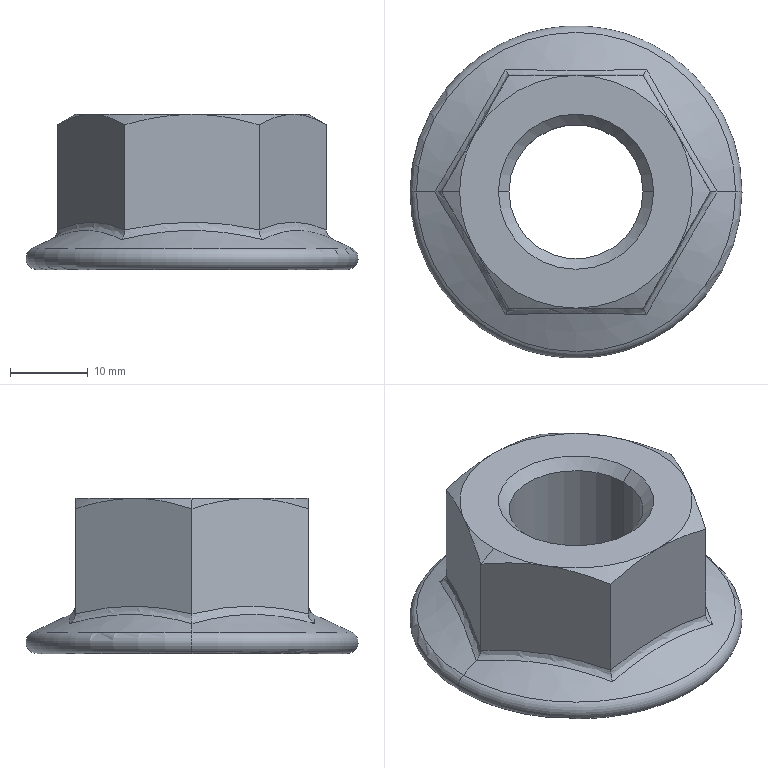Part | SolidWorks | features RevCut 3, Extrusion 1, Fillet 1, LPattern 1, Revolution 1 | 1 solid | 31 faces | box 42.8 x 42.8 x 20 mm | volume 13089 mm3 | cone 13 | plane 8 | spline 6 | torus 2 | cylinder 2 | commonest cylinder face diameters 17.294 x2
STEP:
#1=CARTESIAN_POINT('',(8.647,0.,-18.647));
#2=VERTEX_POINT('',#1);
#3=CARTESIAN_POINT('',(-8.647,0.,-18.647));
#4=VERTEX_POINT('',#3);
#5=CARTESIAN_POINT('',(0.,0.,-18.647));
#6=DIRECTION('',(0.,0.,-1.));
#7=DIRECTION('',(-1.,0.,0.));
#8=AXIS2_PLACEMENT_3D('',#5,#6,#7);
#9=CIRCLE('',#8,8.647);
#10=EDGE_CURVE('',#2,#4,#9,.T.);
#11=ORIENTED_EDGE('',*,*,#10,.F.);
#12=CARTESIAN_POINT('',(10.,0.,-20.));
#13=VERTEX_POINT('',#12);
#14=CARTESIAN_POINT('',(10.,0.,-20.));
#15=DIRECTION('',(0.7071,0.,-0.7071));
#16=VECTOR('',#15,1000.);
#17=LINE('',#14,#16);
#18=EDGE_CURVE('',#2,#13,#17,.T.);
#19=ORIENTED_EDGE('',*,*,#18,.T.);
#20=CARTESIAN_POINT('',(-10.,0.,-20.));
#21=VERTEX_POINT('',#20);
#22=CARTESIAN_POINT('',(0.,0.,-20.));
#23=DIRECTION('',(0.,0.,-1.));
#24=DIRECTION('',(-1.,0.,0.));
#25=AXIS2_PLACEMENT_3D('',#22,#23,#24);
#26=CIRCLE('',#25,10.);
#27=EDGE_CURVE('',#13,#21,#26,.T.);
#28=ORIENTED_EDGE('',*,*,#27,.T.);
#29=CARTESIAN_POINT('',(-10.,0.,-20.));
#30=DIRECTION('',(-0.7071,0.,-0.7071));
#31=VECTOR('',#30,1000.);
#32=LINE('',#29,#31);
#33=EDGE_CURVE('',#4,#21,#32,.T.);
#34=ORIENTED_EDGE('',*,*,#33,.F.);
#35=EDGE_LOOP('',(#11,#19,#28,#34));
#36=FACE_OUTER_BOUND('',#35,.T.);
#37=CARTESIAN_POINT('',(0.,0.,-20.));
#38=DIRECTION('',(0.,0.,-1.));
#39=DIRECTION('',(-1.,0.,0.));
#40=AXIS2_PLACEMENT_3D('',#37,#38,#39);
#41=CONICAL_SURFACE('',#40,10.,0.7854);
#42=ADVANCED_FACE('',(#36),#41,.F.);
#43=CARTESIAN_POINT('',(8.647,0.,-1.353));
#44=VERTEX_POINT('',#43);
#45=CARTESIAN_POINT('',(-8.647,0.,-1.353));
#46=VERTEX_POINT('',#45);
#47=CARTESIAN_POINT('',(0.,0.,-1.353));
#48=DIRECTION('',(0.,0.,-1.));
#49=DIRECTION('',(-1.,0.,0.));
#50=AXIS2_PLACEMENT_3D('',#47,#48,#49);
#51=CIRCLE('',#50,8.647);
#52=EDGE_CURVE('',#44,#46,#51,.T.);
#53=ORIENTED_EDGE('',*,*,#52,.T.);
#54=CARTESIAN_POINT('',(-10.,0.,0.));
#55=VERTEX_POINT('',#54);
#56=CARTESIAN_POINT('',(-8.647,0.,-1.353));
#57=DIRECTION('',(-0.7071,0.,0.7071));
#58=VECTOR('',#57,1000.);
#59=LINE('',#56,#58);
#60=EDGE_CURVE('',#46,#55,#59,.T.);
#61=ORIENTED_EDGE('',*,*,#60,.T.);
#62=CARTESIAN_POINT('',(10.,0.,0.));
#63=VERTEX_POINT('',#62);
#64=CARTESIAN_POINT('',(0.,0.,0.));
#65=DIRECTION('',(0.,0.,-1.));
#66=DIRECTION('',(-1.,0.,0.));
#67=AXIS2_PLACEMENT_3D('',#64,#65,#66);
#68=CIRCLE('',#67,10.);
#69=EDGE_CURVE('',#63,#55,#68,.T.);
#70=ORIENTED_EDGE('',*,*,#69,.F.);
#71=CARTESIAN_POINT('',(8.647,0.,-1.353));
#72=DIRECTION('',(0.7071,0.,0.7071));
#73=VECTOR('',#72,1000.);
#74=LINE('',#71,#73);
#75=EDGE_CURVE('',#44,#63,#74,.T.);
#76=ORIENTED_EDGE('',*,*,#75,.F.);
#77=EDGE_LOOP('',(#53,#61,#70,#76));
#78=FACE_OUTER_BOUND('',#77,.T.);
#79=CARTESIAN_POINT('',(0.,0.,-1.353));
#80=DIRECTION('',(0.,0.,1.));
#81=DIRECTION('',(1.,0.,0.));
#82=AXIS2_PLACEMENT_3D('',#79,#80,#81);
#83=CONICAL_SURFACE('',#82,8.647,0.7854);
#84=ADVANCED_FACE('',(#78),#83,.F.);
#85=CARTESIAN_POINT('',(9.1,15.761,-16.134));
#86=VERTEX_POINT('',#85);
#87=CARTESIAN_POINT('',(18.199,0.,-16.134));
#88=VERTEX_POINT('',#87);
#89=CARTESIAN_POINT('',(9.1,15.761,-16.134));
#90=CARTESIAN_POINT('',(9.83,14.459,-15.778));
#91=CARTESIAN_POINT('',(10.566,13.151,-15.485));
#92=CARTESIAN_POINT('',(12.056,10.52,-15.078));
#93=CARTESIAN_POINT('',(12.811,9.196,-14.966));
#94=CARTESIAN_POINT('',(13.965,7.198,-14.964));
#95=CARTESIAN_POINT('',(14.35,6.534,-14.991));
#96=CARTESIAN_POINT('',(15.123,5.21,-15.097));
#97=CARTESIAN_POINT('',(15.51,4.549,-15.177));
#98=CARTESIAN_POINT('',(16.668,2.582,-15.483));
#99=CARTESIAN_POINT('',(17.436,1.286,-15.778));
#100=CARTESIAN_POINT('',(18.199,0.,-16.134));
#101=B_SPLINE_CURVE_WITH_KNOTS('',3,(#89,#90,#91,#92,#93,#94,#95,#96,#97,#98,#99,#100),.UNSPECIFIED.,.F.,.F.,(4,2,2,2,2,4),(0.,0.004577,0.009154,0.01144,0.01373,0.01831),.UNSPECIFIED.);
#102=EDGE_CURVE('',#86,#88,#101,.T.);
#103=ORIENTED_EDGE('',*,*,#102,.T.);
#104=CARTESIAN_POINT('',(20.563,0.,-17.236));
#105=VERTEX_POINT('',#104);
#106=CARTESIAN_POINT('',(20.563,0.,-17.236));
#107=DIRECTION('',(0.9063,0.,-0.4226));
#108=VECTOR('',#107,1000.);
#109=LINE('',#106,#108);
#110=EDGE_CURVE('',#88,#105,#109,.T.);
#111=ORIENTED_EDGE('',*,*,#110,.T.);
#112=CARTESIAN_POINT('',(-20.563,0.,-17.236));
#113=VERTEX_POINT('',#112);
#114=CARTESIAN_POINT('',(0.,0.,-17.236));
#115=DIRECTION('',(0.,0.,1.));
#116=DIRECTION('',(1.,0.,0.));
#117=AXIS2_PLACEMENT_3D('',#114,#115,#116);
#118=CIRCLE('',#117,20.563);
#119=EDGE_CURVE('',#105,#113,#118,.T.);
#120=ORIENTED_EDGE('',*,*,#119,.T.);
#121=CARTESIAN_POINT('',(-18.199,0.,-16.134));
#122=VERTEX_POINT('',#121);
#123=CARTESIAN_POINT('',(-20.563,0.,-17.236));
#124=DIRECTION('',(-0.9063,0.,-0.4226));
#125=VECTOR('',#124,1000.);
#126=LINE('',#123,#125);
#127=EDGE_CURVE('',#122,#113,#126,.T.);
#128=ORIENTED_EDGE('',*,*,#127,.F.);
#129=CARTESIAN_POINT('',(-9.1,15.761,-16.134));
#130=VERTEX_POINT('',#129);
#131=CARTESIAN_POINT('',(-18.199,0.,-16.134));
#132=CARTESIAN_POINT('',(-17.437,1.284,-15.778));
#133=CARTESIAN_POINT('',(-16.672,2.575,-15.485));
#134=CARTESIAN_POINT('',(-15.138,5.181,-15.078));
#135=CARTESIAN_POINT('',(-14.37,6.497,-14.966));
#136=CARTESIAN_POINT('',(-13.216,8.495,-14.964));
#137=CARTESIAN_POINT('',(-12.834,9.161,-14.991));
#138=CARTESIAN_POINT('',(-12.073,10.492,-15.097));
#139=CARTESIAN_POINT('',(-11.695,11.157,-15.177));
#140=CARTESIAN_POINT('',(-10.57,13.144,-15.483));
#141=CARTESIAN_POINT('',(-9.832,14.457,-15.778));
#142=CARTESIAN_POINT('',(-9.1,15.761,-16.134));
#143=B_SPLINE_CURVE_WITH_KNOTS('',3,(#131,#132,#133,#134,#135,#136,#137,#138,#139,#140,#141,#142),.UNSPECIFIED.,.F.,.F.,(4,2,2,2,2,4),(0.,0.004577,0.009154,0.01144,0.01373,0.01831),.UNSPECIFIED.);
#144=EDGE_CURVE('',#122,#130,#143,.T.);
#145=ORIENTED_EDGE('',*,*,#144,.T.);
#146=CARTESIAN_POINT('',(-9.1,15.761,-16.134));
#147=CARTESIAN_POINT('',(-7.607,15.743,-15.778));
#148=CARTESIAN_POINT('',(-6.106,15.726,-15.485));
#149=CARTESIAN_POINT('',(-3.082,15.701,-15.078));
#150=CARTESIAN_POINT('',(-1.558,15.693,-14.966));
#151=CARTESIAN_POINT('',(0.749,15.693,-14.964));
#152=CARTESIAN_POINT('',(1.517,15.695,-14.991));
#153=CARTESIAN_POINT('',(3.05,15.702,-15.098));
#154=CARTESIAN_POINT('',(3.815,15.707,-15.177));
#155=CARTESIAN_POINT('',(6.098,15.726,-15.483));
#156=CARTESIAN_POINT('',(7.604,15.743,-15.778));
#157=CARTESIAN_POINT('',(9.1,15.761,-16.134));
#158=B_SPLINE_CURVE_WITH_KNOTS('',3,(#146,#147,#148,#149,#150,#151,#152,#153,#154,#155,#156,#157),.UNSPECIFIED.,.F.,.F.,(4,2,2,2,2,4),(0.,0.004577,0.009155,0.01144,0.01373,0.01831),.UNSPECIFIED.);
#159=EDGE_CURVE('',#130,#86,#158,.T.);
#160=ORIENTED_EDGE('',*,*,#159,.T.);
#161=EDGE_LOOP('',(#103,#111,#120,#128,#145,#160));
#162=FACE_OUTER_BOUND('',#161,.T.);
#163=CARTESIAN_POINT('',(0.,0.,-17.236));
#164=DIRECTION('',(0.,0.,-1.));
#165=DIRECTION('',(-1.,0.,0.));
#166=AXIS2_PLACEMENT_3D('',#163,#164,#165);
#167=CONICAL_SURFACE('',#166,20.563,1.134);
#168=ADVANCED_FACE('',(#162),#167,.T.);
#169=CARTESIAN_POINT('',(19.95,0.,-20.));
#170=VERTEX_POINT('',#169);
#171=CARTESIAN_POINT('',(-19.95,0.,-20.));
#172=VERTEX_POINT('',#171);
#173=CARTESIAN_POINT('',(0.,0.,-20.));
#174=DIRECTION('',(0.,0.,1.));
#175=DIRECTION('',(1.,0.,0.));
#176=AXIS2_PLACEMENT_3D('',#173,#174,#175);
#177=CIRCLE('',#176,19.95);
#178=EDGE_CURVE('',#170,#172,#177,.T.);
#179=ORIENTED_EDGE('',*,*,#178,.T.);
#180=CARTESIAN_POINT('',(-19.95,0.,-18.55));
#181=DIRECTION('',(0.,1.,0.));
#182=DIRECTION('',(-1.,0.,0.));
#183=AXIS2_PLACEMENT_3D('',#180,#181,#182);
#184=CIRCLE('',#183,1.45);
#185=EDGE_CURVE('',#172,#113,#184,.T.);
#186=ORIENTED_EDGE('',*,*,#185,.T.);
#187=ORIENTED_EDGE('',*,*,#119,.F.);
#188=CARTESIAN_POINT('',(19.95,0.,-18.55));
#189=DIRECTION('',(0.,-1.,0.));
#190=DIRECTION('',(0.,0.,-1.));
#191=AXIS2_PLACEMENT_3D('',#188,#189,#190);
#192=CIRCLE('',#191,1.45);
#193=EDGE_CURVE('',#170,#105,#192,.T.);
#194=ORIENTED_EDGE('',*,*,#193,.F.);
#195=EDGE_LOOP('',(#179,#186,#187,#194));
#196=FACE_OUTER_BOUND('',#195,.T.);
#197=CARTESIAN_POINT('',(0.,0.,-18.55));
#198=DIRECTION('',(0.,0.,1.));
#199=DIRECTION('',(1.,0.,0.));
#200=AXIS2_PLACEMENT_3D('',#197,#198,#199);
#201=TOROIDAL_SURFACE('',#200,19.95,1.45);
#202=ADVANCED_FACE('',(#196),#201,.T.);
#203=CARTESIAN_POINT('',(-15.,0.,0.));
#204=VERTEX_POINT('',#203);
#205=CARTESIAN_POINT('',(-12.99,-7.5,0.));
#206=VERTEX_POINT('',#205);
#207=CARTESIAN_POINT('',(0.,0.,0.));
#208=DIRECTION('',(0.,0.,1.));
#209=DIRECTION('',(-1.,0.,0.));
#210=AXIS2_PLACEMENT_3D('',#207,#208,#209);
#211=CIRCLE('',#210,15.);
#212=EDGE_CURVE('',#204,#206,#211,.T.);
#213=ORIENTED_EDGE('',*,*,#212,.F.);
#214=CARTESIAN_POINT('',(-17.321,0.,-1.34));
#215=VERTEX_POINT('',#214);
#216=CARTESIAN_POINT('',(-15.,0.,0.));
#217=DIRECTION('',(-0.866,0.,-0.5));
#218=VECTOR('',#217,1000.);
#219=LINE('',#216,#218);
#220=EDGE_CURVE('',#204,#215,#219,.T.);
#221=ORIENTED_EDGE('',*,*,#220,.T.);
#222=CARTESIAN_POINT('',(-17.321,0.,-1.34));
#223=CARTESIAN_POINT('',(-16.612,-1.227,-0.9308));
#224=CARTESIAN_POINT('',(-15.899,-2.463,-0.5939));
#225=CARTESIAN_POINT('',(-14.457,-4.96,-0.1277));
#226=CARTESIAN_POINT('',(-13.728,-6.222,0.));
#227=CARTESIAN_POINT('',(-12.99,-7.5,0.));
#228=B_SPLINE_CURVE_WITH_KNOTS('',3,(#222,#223,#224,#225,#226,#227),.UNSPECIFIED.,.F.,.F.,(4,2,4),(0.000000238,0.004382,0.008763),.UNSPECIFIED.);
#229=EDGE_CURVE('',#215,#206,#228,.T.);
#230=ORIENTED_EDGE('',*,*,#229,.T.);
#231=EDGE_LOOP('',(#213,#221,#230));
#232=FACE_OUTER_BOUND('',#231,.T.);
#233=CARTESIAN_POINT('',(0.,0.,0.));
#234=DIRECTION('',(0.,0.,-1.));
#235=DIRECTION('',(-1.,0.,0.));
#236=AXIS2_PLACEMENT_3D('',#233,#234,#235);
#237=CONICAL_SURFACE('',#236,15.,1.047);
#238=ADVANCED_FACE('',(#232),#237,.T.);
#239=ORIENTED_EDGE('',*,*,#10,.T.);
#240=CARTESIAN_POINT('',(-8.647,0.,-20.));
#241=DIRECTION('',(0.,0.,1.));
#242=VECTOR('',#241,1000.);
#243=LINE('',#240,#242);
#244=EDGE_CURVE('',#4,#46,#243,.T.);
#245=ORIENTED_EDGE('',*,*,#244,.T.);
#246=ORIENTED_EDGE('',*,*,#52,.F.);
#247=CARTESIAN_POINT('',(8.647,0.,-20.));
#248=DIRECTION('',(0.,0.,1.));
#249=VECTOR('',#248,1000.);
#250=LINE('',#247,#249);
#251=EDGE_CURVE('',#2,#44,#250,.T.);
#252=ORIENTED_EDGE('',*,*,#251,.F.);
#253=EDGE_LOOP('',(#239,#245,#246,#252));
#254=FACE_OUTER_BOUND('',#253,.T.);
#255=CARTESIAN_POINT('',(0.,0.,-20.));
#256=DIRECTION('',(0.,0.,1.));
#257=DIRECTION('',(1.,0.,0.));
#258=AXIS2_PLACEMENT_3D('',#255,#256,#257);
#259=CYLINDRICAL_SURFACE('',#258,8.647);
#260=ADVANCED_FACE('',(#254),#259,.F.);
#261=CARTESIAN_POINT('',(-8.66,-15.,-14.889));
#262=VERTEX_POINT('',#261);
#263=CARTESIAN_POINT('',(-8.66,-15.,-1.34));
#264=VERTEX_POINT('',#263);
#265=CARTESIAN_POINT('',(-8.66,-15.,-20.));
#266=DIRECTION('',(0.,0.,1.));
#267=VECTOR('',#266,1000.);
#268=LINE('',#265,#267);
#269=EDGE_CURVE('',#262,#264,#268,.T.);
#270=ORIENTED_EDGE('',*,*,#269,.F.);
#271=CARTESIAN_POINT('',(8.66,-15.,-14.889));
#272=VERTEX_POINT('',#271);
#273=CARTESIAN_POINT('',(-8.66,-15.,-14.889));
#274=CARTESIAN_POINT('',(-7.234,-15.,-14.575));
#275=CARTESIAN_POINT('',(-5.801,-15.,-14.321));
#276=CARTESIAN_POINT('',(-2.915,-15.,-13.971));
#277=CARTESIAN_POINT('',(-1.463,-15.,-13.877));
#278=CARTESIAN_POINT('',(1.463,-15.,-13.877));
#279=CARTESIAN_POINT('',(2.915,-15.,-13.971));
#280=CARTESIAN_POINT('',(5.801,-15.,-14.321));
#281=CARTESIAN_POINT('',(7.234,-15.,-14.575));
#282=CARTESIAN_POINT('',(8.66,-15.,-14.889));
#283=B_SPLINE_CURVE_WITH_KNOTS('',3,(#273,#274,#275,#276,#277,#278,#279,#280,#281,#282),.UNSPECIFIED.,.F.,.F.,(4,2,2,2,4),(0.,0.00436,0.008719,0.01308,0.01744),.UNSPECIFIED.);
#284=EDGE_CURVE('',#262,#272,#283,.T.);
#285=ORIENTED_EDGE('',*,*,#284,.T.);
#286=CARTESIAN_POINT('',(8.66,-15.,-1.34));
#287=VERTEX_POINT('',#286);
#288=CARTESIAN_POINT('',(8.66,-15.,-20.));
#289=DIRECTION('',(0.,0.,1.));
#290=VECTOR('',#289,1000.);
#291=LINE('',#288,#290);
#292=EDGE_CURVE('',#272,#287,#291,.T.);
#293=ORIENTED_EDGE('',*,*,#292,.T.);
#294=CARTESIAN_POINT('',(0.,-15.,0.));
#295=VERTEX_POINT('',#294);
#296=CARTESIAN_POINT('',(0.,-15.,0.));
#297=CARTESIAN_POINT('',(0.7322,-15.,0.));
#298=CARTESIAN_POINT('',(1.467,-15.,-0.03111));
#299=CARTESIAN_POINT('',(2.94,-15.,-0.1548));
#300=CARTESIAN_POINT('',(3.672,-15.,-0.2467));
#301=CARTESIAN_POINT('',(5.841,-15.,-0.5989));
#302=CARTESIAN_POINT('',(7.26,-15.,-0.9355));
#303=CARTESIAN_POINT('',(8.66,-15.,-1.34));
#304=B_SPLINE_CURVE_WITH_KNOTS('',3,(#296,#297,#298,#299,#300,#301,#302,#303),.UNSPECIFIED.,.F.,.F.,(4,2,2,4),(0.02421,0.0264,0.0286,0.03298),.UNSPECIFIED.);
#305=EDGE_CURVE('',#295,#287,#304,.T.);
#306=ORIENTED_EDGE('',*,*,#305,.F.);
#307=CARTESIAN_POINT('',(-8.66,-15.,-1.34));
#308=CARTESIAN_POINT('',(-7.956,-15.,-1.136));
#309=CARTESIAN_POINT('',(-7.245,-15.,-0.9498));
#310=CARTESIAN_POINT('',(-5.807,-15.,-0.6186));
#311=CARTESIAN_POINT('',(-5.086,-15.,-0.4755));
#312=CARTESIAN_POINT('',(-2.917,-15.,-0.1258));
#313=CARTESIAN_POINT('',(-1.463,-15.,0.));
#314=CARTESIAN_POINT('',(0.,-15.,0.));
#315=B_SPLINE_CURVE_WITH_KNOTS('',3,(#307,#308,#309,#310,#311,#312,#313,#314),.UNSPECIFIED.,.F.,.F.,(4,2,2,4),(0.01545,0.01764,0.01983,0.02421),.UNSPECIFIED.);
#316=EDGE_CURVE('',#264,#295,#315,.T.);
#317=ORIENTED_EDGE('',*,*,#316,.F.);
#318=EDGE_LOOP('',(#270,#285,#293,#306,#317));
#319=FACE_OUTER_BOUND('',#318,.T.);
#320=CARTESIAN_POINT('',(-8.66,-15.,-20.));
#321=DIRECTION('',(0.,-1.,0.));
#322=DIRECTION('',(1.,0.,0.));
#323=AXIS2_PLACEMENT_3D('',#320,#321,#322);
#324=PLANE('',#323);
#325=ADVANCED_FACE('',(#319),#324,.T.);
#326=CARTESIAN_POINT('',(-17.321,0.,-14.889));
#327=VERTEX_POINT('',#326);
#328=CARTESIAN_POINT('',(-17.321,0.,-20.));
#329=DIRECTION('',(0.,0.,1.));
#330=VECTOR('',#329,1000.);
#331=LINE('',#328,#330);
#332=EDGE_CURVE('',#327,#215,#331,.T.);
#333=ORIENTED_EDGE('',*,*,#332,.F.);
#334=CARTESIAN_POINT('',(-17.321,0.,-14.889));
#335=CARTESIAN_POINT('',(-16.607,-1.235,-14.575));
#336=CARTESIAN_POINT('',(-15.891,-2.477,-14.321));
#337=CARTESIAN_POINT('',(-14.448,-4.976,-13.971));
#338=CARTESIAN_POINT('',(-13.722,-6.234,-13.877));
#339=CARTESIAN_POINT('',(-12.259,-8.767,-13.877));
#340=CARTESIAN_POINT('',(-11.533,-10.025,-13.971));
#341=CARTESIAN_POINT('',(-10.09,-12.523,-14.321));
#342=CARTESIAN_POINT('',(-9.373,-13.765,-14.575));
#343=CARTESIAN_POINT('',(-8.66,-15.,-14.889));
#344=B_SPLINE_CURVE_WITH_KNOTS('',3,(#334,#335,#336,#337,#338,#339,#340,#341,#342,#343),.UNSPECIFIED.,.F.,.F.,(4,2,2,2,4),(0.,0.00436,0.00872,0.01308,0.01744),.UNSPECIFIED.);
#345=EDGE_CURVE('',#327,#262,#344,.T.);
#346=ORIENTED_EDGE('',*,*,#345,.T.);
#347=ORIENTED_EDGE('',*,*,#269,.T.);
#348=CARTESIAN_POINT('',(-12.99,-7.5,0.));
#349=CARTESIAN_POINT('',(-12.623,-8.136,0.));
#350=CARTESIAN_POINT('',(-12.254,-8.776,-0.03167));
#351=CARTESIAN_POINT('',(-11.524,-10.041,-0.1542));
#352=CARTESIAN_POINT('',(-11.161,-10.669,-0.245));
#353=CARTESIAN_POINT('',(-10.079,-12.542,-0.595));
#354=CARTESIAN_POINT('',(-9.367,-13.776,-0.9318));
#355=CARTESIAN_POINT('',(-8.66,-15.,-1.34));
#356=B_SPLINE_CURVE_WITH_KNOTS('',3,(#348,#349,#350,#351,#352,#353,#354,#355),.UNSPECIFIED.,.F.,.F.,(4,2,2,4),(0.008763,0.01095,0.01313,0.01749),.UNSPECIFIED.);
#357=EDGE_CURVE('',#206,#264,#356,.T.);
#358=ORIENTED_EDGE('',*,*,#357,.F.);
#359=ORIENTED_EDGE('',*,*,#229,.F.);
#360=EDGE_LOOP('',(#333,#346,#347,#358,#359));
#361=FACE_OUTER_BOUND('',#360,.T.);
#362=CARTESIAN_POINT('',(-17.321,0.,-20.));
#363=DIRECTION('',(-0.866,-0.5,0.));
#364=DIRECTION('',(0.5,-0.866,0.));
#365=AXIS2_PLACEMENT_3D('',#362,#363,#364);
#366=PLANE('',#365);
#367=ADVANCED_FACE('',(#361),#366,.T.);
#368=CARTESIAN_POINT('',(-8.66,15.,-14.889));
#369=VERTEX_POINT('',#368);
#370=CARTESIAN_POINT('',(-8.66,15.,-1.34));
#371=VERTEX_POINT('',#370);
#372=CARTESIAN_POINT('',(-8.66,15.,-20.));
#373=DIRECTION('',(0.,0.,1.));
#374=VECTOR('',#373,1000.);
#375=LINE('',#372,#374);
#376=EDGE_CURVE('',#369,#371,#375,.T.);
#377=ORIENTED_EDGE('',*,*,#376,.F.);
#378=CARTESIAN_POINT('',(-8.66,15.,-14.889));
#379=CARTESIAN_POINT('',(-9.373,13.765,-14.575));
#380=CARTESIAN_POINT('',(-10.09,12.523,-14.321));
#381=CARTESIAN_POINT('',(-11.533,10.024,-13.971));
#382=CARTESIAN_POINT('',(-12.259,8.766,-13.877));
#383=CARTESIAN_POINT('',(-13.722,6.233,-13.877));
#384=CARTESIAN_POINT('',(-14.448,4.975,-13.971));
#385=CARTESIAN_POINT('',(-15.891,2.477,-14.321));
#386=CARTESIAN_POINT('',(-16.607,1.235,-14.575));
#387=CARTESIAN_POINT('',(-17.321,0.,-14.889));
#388=B_SPLINE_CURVE_WITH_KNOTS('',3,(#378,#379,#380,#381,#382,#383,#384,#385,#386,#387),.UNSPECIFIED.,.F.,.F.,(4,2,2,2,4),(0.,0.00436,0.00872,0.01308,0.01744),.UNSPECIFIED.);
#389=EDGE_CURVE('',#369,#327,#388,.T.);
#390=ORIENTED_EDGE('',*,*,#389,.T.);
#391=ORIENTED_EDGE('',*,*,#332,.T.);
#392=CARTESIAN_POINT('',(-12.99,7.5,0.));
#393=VERTEX_POINT('',#392);
#394=CARTESIAN_POINT('',(-12.99,7.5,0.));
#395=CARTESIAN_POINT('',(-13.358,6.864,0.));
#396=CARTESIAN_POINT('',(-13.727,6.224,-0.03167));
#397=CARTESIAN_POINT('',(-14.457,4.959,-0.1542));
#398=CARTESIAN_POINT('',(-14.82,4.331,-0.245));
#399=CARTESIAN_POINT('',(-15.901,2.458,-0.595));
#400=CARTESIAN_POINT('',(-16.614,1.224,-0.9318));
#401=CARTESIAN_POINT('',(-17.321,0.,-1.34));
#402=B_SPLINE_CURVE_WITH_KNOTS('',3,(#394,#395,#396,#397,#398,#399,#400,#401),.UNSPECIFIED.,.F.,.F.,(4,2,2,4),(0.008763,0.01095,0.01313,0.01749),.UNSPECIFIED.);
#403=EDGE_CURVE('',#393,#215,#402,.T.);
#404=ORIENTED_EDGE('',*,*,#403,.F.);
#405=CARTESIAN_POINT('',(-8.66,15.,-1.34));
#406=CARTESIAN_POINT('',(-9.369,13.773,-0.9308));
#407=CARTESIAN_POINT('',(-10.082,12.537,-0.5939));
#408=CARTESIAN_POINT('',(-11.524,10.04,-0.1277));
#409=CARTESIAN_POINT('',(-12.253,8.778,0.));
#410=CARTESIAN_POINT('',(-12.99,7.5,0.));
#411=B_SPLINE_CURVE_WITH_KNOTS('',3,(#405,#406,#407,#408,#409,#410),.UNSPECIFIED.,.F.,.F.,(4,2,4),(0.000000238,0.004382,0.008763),.UNSPECIFIED.);
#412=EDGE_CURVE('',#371,#393,#411,.T.);
#413=ORIENTED_EDGE('',*,*,#412,.F.);
#414=EDGE_LOOP('',(#377,#390,#391,#404,#413));
#415=FACE_OUTER_BOUND('',#414,.T.);
#416=CARTESIAN_POINT('',(-8.66,15.,-20.));
#417=DIRECTION('',(-0.866,0.5,0.));
#418=DIRECTION('',(-0.5,-0.866,0.));
#419=AXIS2_PLACEMENT_3D('',#416,#417,#418);
#420=PLANE('',#419);
#421=ADVANCED_FACE('',(#415),#420,.T.);
#422=CARTESIAN_POINT('',(8.66,15.,-14.889));
#423=VERTEX_POINT('',#422);
#424=CARTESIAN_POINT('',(8.66,15.,-1.34));
#425=VERTEX_POINT('',#424);
#426=CARTESIAN_POINT('',(8.66,15.,-20.));
#427=DIRECTION('',(0.,0.,1.));
#428=VECTOR('',#427,1000.);
#429=LINE('',#426,#428);
#430=EDGE_CURVE('',#423,#425,#429,.T.);
#431=ORIENTED_EDGE('',*,*,#430,.F.);
#432=CARTESIAN_POINT('',(8.66,15.,-14.889));
#433=CARTESIAN_POINT('',(7.234,15.,-14.575));
#434=CARTESIAN_POINT('',(5.801,15.,-14.321));
#435=CARTESIAN_POINT('',(2.915,15.,-13.971));
#436=CARTESIAN_POINT('',(1.463,15.,-13.877));
#437=CARTESIAN_POINT('',(-1.463,15.,-13.877));
#438=CARTESIAN_POINT('',(-2.915,15.,-13.971));
#439=CARTESIAN_POINT('',(-5.801,15.,-14.321));
#440=CARTESIAN_POINT('',(-7.234,15.,-14.575));
#441=CARTESIAN_POINT('',(-8.66,15.,-14.889));
#442=B_SPLINE_CURVE_WITH_KNOTS('',3,(#432,#433,#434,#435,#436,#437,#438,#439,#440,#441),.UNSPECIFIED.,.F.,.F.,(4,2,2,2,4),(0.,0.00436,0.008719,0.01308,0.01744),.UNSPECIFIED.);
#443=EDGE_CURVE('',#423,#369,#442,.T.);
#444=ORIENTED_EDGE('',*,*,#443,.T.);
#445=ORIENTED_EDGE('',*,*,#376,.T.);
#446=CARTESIAN_POINT('',(0.,15.,0.));
#447=VERTEX_POINT('',#446);
#448=CARTESIAN_POINT('',(0.,15.,0.));
#449=CARTESIAN_POINT('',(-1.463,15.,0.));
#450=CARTESIAN_POINT('',(-2.917,15.,-0.1258));
#451=CARTESIAN_POINT('',(-5.086,15.,-0.4755));
#452=CARTESIAN_POINT('',(-5.807,15.,-0.6186));
#453=CARTESIAN_POINT('',(-7.245,15.,-0.9498));
#454=CARTESIAN_POINT('',(-7.956,15.,-1.136));
#455=CARTESIAN_POINT('',(-8.66,15.,-1.34));
#456=B_SPLINE_CURVE_WITH_KNOTS('',3,(#448,#449,#450,#451,#452,#453,#454,#455),.UNSPECIFIED.,.F.,.F.,(4,2,2,4),(0.01509,0.01946,0.02165,0.02383),.UNSPECIFIED.);
#457=EDGE_CURVE('',#447,#371,#456,.T.);
#458=ORIENTED_EDGE('',*,*,#457,.F.);
#459=CARTESIAN_POINT('',(8.66,15.,-1.34));
#460=CARTESIAN_POINT('',(7.26,15.,-0.9355));
#461=CARTESIAN_POINT('',(5.841,15.,-0.5989));
#462=CARTESIAN_POINT('',(3.672,15.,-0.2467));
#463=CARTESIAN_POINT('',(2.94,15.,-0.1548));
#464=CARTESIAN_POINT('',(1.467,15.,-0.03111));
#465=CARTESIAN_POINT('',(0.7322,15.,0.));
#466=CARTESIAN_POINT('',(0.,15.,0.));
#467=B_SPLINE_CURVE_WITH_KNOTS('',3,(#459,#460,#461,#462,#463,#464,#465,#466),.UNSPECIFIED.,.F.,.F.,(4,2,2,4),(0.006348,0.01072,0.01291,0.01509),.UNSPECIFIED.);
#468=EDGE_CURVE('',#425,#447,#467,.T.);
#469=ORIENTED_EDGE('',*,*,#468,.F.);
#470=EDGE_LOOP('',(#431,#444,#445,#458,#469));
#471=FACE_OUTER_BOUND('',#470,.T.);
#472=CARTESIAN_POINT('',(8.66,15.,-20.));
#473=DIRECTION('',(0.,1.,0.));
#474=DIRECTION('',(-1.,0.,0.));
#475=AXIS2_PLACEMENT_3D('',#472,#473,#474);
#476=PLANE('',#475);
#477=ADVANCED_FACE('',(#471),#476,.T.);
#478=CARTESIAN_POINT('',(17.321,0.,-14.889));
#479=VERTEX_POINT('',#478);
#480=CARTESIAN_POINT('',(17.321,0.,-1.34));
#481=VERTEX_POINT('',#480);
#482=CARTESIAN_POINT('',(17.321,0.,-20.));
#483=DIRECTION('',(0.,0.,1.));
#484=VECTOR('',#483,1000.);
#485=LINE('',#482,#484);
#486=EDGE_CURVE('',#479,#481,#485,.T.);
#487=ORIENTED_EDGE('',*,*,#486,.F.);
#488=CARTESIAN_POINT('',(17.321,0.,-14.889));
#489=CARTESIAN_POINT('',(16.607,1.235,-14.575));
#490=CARTESIAN_POINT('',(15.891,2.477,-14.321));
#491=CARTESIAN_POINT('',(14.448,4.976,-13.971));
#492=CARTESIAN_POINT('',(13.722,6.234,-13.877));
#493=CARTESIAN_POINT('',(12.259,8.767,-13.877));
#494=CARTESIAN_POINT('',(11.533,10.025,-13.971));
#495=CARTESIAN_POINT('',(10.09,12.523,-14.321));
#496=CARTESIAN_POINT('',(9.373,13.765,-14.575));
#497=CARTESIAN_POINT('',(8.66,15.,-14.889));
#498=B_SPLINE_CURVE_WITH_KNOTS('',3,(#488,#489,#490,#491,#492,#493,#494,#495,#496,#497),.UNSPECIFIED.,.F.,.F.,(4,2,2,2,4),(0.,0.00436,0.00872,0.01308,0.01744),.UNSPECIFIED.);
#499=EDGE_CURVE('',#479,#423,#498,.T.);
#500=ORIENTED_EDGE('',*,*,#499,.T.);
#501=ORIENTED_EDGE('',*,*,#430,.T.);
#502=CARTESIAN_POINT('',(12.99,7.5,0.));
#503=VERTEX_POINT('',#502);
#504=CARTESIAN_POINT('',(12.99,7.5,0.));
#505=CARTESIAN_POINT('',(12.623,8.136,0.));
#506=CARTESIAN_POINT('',(12.254,8.776,-0.03167));
#507=CARTESIAN_POINT('',(11.524,10.041,-0.1542));
#508=CARTESIAN_POINT('',(11.161,10.669,-0.245));
#509=CARTESIAN_POINT('',(10.079,12.542,-0.595));
#510=CARTESIAN_POINT('',(9.367,13.776,-0.9318));
#511=CARTESIAN_POINT('',(8.66,15.,-1.34));
#512=B_SPLINE_CURVE_WITH_KNOTS('',3,(#504,#505,#506,#507,#508,#509,#510,#511),.UNSPECIFIED.,.F.,.F.,(4,2,2,4),(0.008763,0.01095,0.01313,0.01749),.UNSPECIFIED.);
#513=EDGE_CURVE('',#503,#425,#512,.T.);
#514=ORIENTED_EDGE('',*,*,#513,.F.);
#515=CARTESIAN_POINT('',(17.321,0.,-1.34));
#516=CARTESIAN_POINT('',(16.612,1.227,-0.9308));
#517=CARTESIAN_POINT('',(15.899,2.463,-0.5939));
#518=CARTESIAN_POINT('',(14.457,4.96,-0.1277));
#519=CARTESIAN_POINT('',(13.728,6.222,0.));
#520=CARTESIAN_POINT('',(12.99,7.5,0.));
#521=B_SPLINE_CURVE_WITH_KNOTS('',3,(#515,#516,#517,#518,#519,#520),.UNSPECIFIED.,.F.,.F.,(4,2,4),(0.000000238,0.004382,0.008763),.UNSPECIFIED.);
#522=EDGE_CURVE('',#481,#503,#521,.T.);
#523=ORIENTED_EDGE('',*,*,#522,.F.);
#524=EDGE_LOOP('',(#487,#500,#501,#514,#523));
#525=FACE_OUTER_BOUND('',#524,.T.);
#526=CARTESIAN_POINT('',(17.321,0.,-20.));
#527=DIRECTION('',(0.866,0.5,0.));
#528=DIRECTION('',(-0.5,0.866,0.));
#529=AXIS2_PLACEMENT_3D('',#526,#527,#528);
#530=PLANE('',#529);
#531=ADVANCED_FACE('',(#525),#530,.T.);
#532=ORIENTED_EDGE('',*,*,#292,.F.);
#533=CARTESIAN_POINT('',(8.66,-15.,-14.889));
#534=CARTESIAN_POINT('',(9.373,-13.765,-14.575));
#535=CARTESIAN_POINT('',(10.09,-12.523,-14.321));
#536=CARTESIAN_POINT('',(11.533,-10.024,-13.971));
#537=CARTESIAN_POINT('',(12.259,-8.766,-13.877));
#538=CARTESIAN_POINT('',(13.722,-6.233,-13.877));
#539=CARTESIAN_POINT('',(14.448,-4.975,-13.971));
#540=CARTESIAN_POINT('',(15.891,-2.477,-14.321));
#541=CARTESIAN_POINT('',(16.607,-1.235,-14.575));
#542=CARTESIAN_POINT('',(17.321,0.,-14.889));
#543=B_SPLINE_CURVE_WITH_KNOTS('',3,(#533,#534,#535,#536,#537,#538,#539,#540,#541,#542),.UNSPECIFIED.,.F.,.F.,(4,2,2,2,4),(0.,0.00436,0.00872,0.01308,0.01744),.UNSPECIFIED.);
#544=EDGE_CURVE('',#272,#479,#543,.T.);
#545=ORIENTED_EDGE('',*,*,#544,.T.);
#546=ORIENTED_EDGE('',*,*,#486,.T.);
#547=CARTESIAN_POINT('',(12.99,-7.5,0.));
#548=VERTEX_POINT('',#547);
#549=CARTESIAN_POINT('',(12.99,-7.5,0.));
#550=CARTESIAN_POINT('',(13.358,-6.864,0.));
#551=CARTESIAN_POINT('',(13.727,-6.224,-0.03167));
#552=CARTESIAN_POINT('',(14.457,-4.959,-0.1542));
#553=CARTESIAN_POINT('',(14.82,-4.331,-0.245));
#554=CARTESIAN_POINT('',(15.901,-2.458,-0.595));
#555=CARTESIAN_POINT('',(16.614,-1.224,-0.9318));
#556=CARTESIAN_POINT('',(17.321,0.,-1.34));
#557=B_SPLINE_CURVE_WITH_KNOTS('',3,(#549,#550,#551,#552,#553,#554,#555,#556),.UNSPECIFIED.,.F.,.F.,(4,2,2,4),(0.008763,0.01095,0.01313,0.01749),.UNSPECIFIED.);
#558=EDGE_CURVE('',#548,#481,#557,.T.);
#559=ORIENTED_EDGE('',*,*,#558,.F.);
#560=CARTESIAN_POINT('',(8.66,-15.,-1.34));
#561=CARTESIAN_POINT('',(9.369,-13.773,-0.9308));
#562=CARTESIAN_POINT('',(10.082,-12.537,-0.5939));
#563=CARTESIAN_POINT('',(11.524,-10.04,-0.1277));
#564=CARTESIAN_POINT('',(12.253,-8.778,0.));
#565=CARTESIAN_POINT('',(12.99,-7.5,0.));
#566=B_SPLINE_CURVE_WITH_KNOTS('',3,(#560,#561,#562,#563,#564,#565),.UNSPECIFIED.,.F.,.F.,(4,2,4),(0.000000238,0.004382,0.008763),.UNSPECIFIED.);
#567=EDGE_CURVE('',#287,#548,#566,.T.);
#568=ORIENTED_EDGE('',*,*,#567,.F.);
#569=EDGE_LOOP('',(#532,#545,#546,#559,#568));
#570=FACE_OUTER_BOUND('',#569,.T.);
#571=CARTESIAN_POINT('',(8.66,-15.,-20.));
#572=DIRECTION('',(0.866,-0.5,0.));
#573=DIRECTION('',(0.5,0.866,0.));
#574=AXIS2_PLACEMENT_3D('',#571,#572,#573);
#575=PLANE('',#574);
#576=ADVANCED_FACE('',(#570),#575,.T.);
#577=CARTESIAN_POINT('',(0.,0.,-20.));
#578=DIRECTION('',(0.,0.,-1.));
#579=DIRECTION('',(-1.,0.,0.));
#580=AXIS2_PLACEMENT_3D('',#577,#578,#579);
#581=CIRCLE('',#580,10.);
#582=EDGE_CURVE('',#21,#13,#581,.T.);
#583=ORIENTED_EDGE('',*,*,#582,.F.);
#584=ORIENTED_EDGE('',*,*,#27,.F.);
#585=EDGE_LOOP('',(#583,#584));
#586=FACE_BOUND('',#585,.T.);
#587=ORIENTED_EDGE('',*,*,#178,.F.);
#588=CARTESIAN_POINT('',(0.,0.,-20.));
#589=DIRECTION('',(0.,0.,1.));
#590=DIRECTION('',(1.,0.,0.));
#591=AXIS2_PLACEMENT_3D('',#588,#589,#590);
#592=CIRCLE('',#591,19.95);
#593=EDGE_CURVE('',#172,#170,#592,.T.);
#594=ORIENTED_EDGE('',*,*,#593,.F.);
#595=EDGE_LOOP('',(#587,#594));
#596=FACE_OUTER_BOUND('',#595,.T.);
#597=CARTESIAN_POINT('',(-25.981,-15.,-20.));
#598=DIRECTION('',(0.,0.,-1.));
#599=DIRECTION('',(-1.,0.,0.));
#600=AXIS2_PLACEMENT_3D('',#597,#598,#599);
#601=PLANE('',#600);
#602=ADVANCED_FACE('',(#586,#596),#601,.T.);
#603=ORIENTED_EDGE('',*,*,#69,.T.);
#604=CARTESIAN_POINT('',(0.,0.,0.));
#605=DIRECTION('',(0.,0.,-1.));
#606=DIRECTION('',(-1.,0.,0.));
#607=AXIS2_PLACEMENT_3D('',#604,#605,#606);
#608=CIRCLE('',#607,10.);
#609=EDGE_CURVE('',#55,#63,#608,.T.);
#610=ORIENTED_EDGE('',*,*,#609,.T.);
#611=EDGE_LOOP('',(#603,#610));
#612=FACE_BOUND('',#611,.T.);
#613=CARTESIAN_POINT('',(0.,0.,0.));
#614=DIRECTION('',(0.,0.,1.));
#615=DIRECTION('',(-1.,0.,0.));
#616=AXIS2_PLACEMENT_3D('',#613,#614,#615);
#617=CIRCLE('',#616,15.);
#618=EDGE_CURVE('',#393,#204,#617,.T.);
#619=ORIENTED_EDGE('',*,*,#618,.T.);
#620=ORIENTED_EDGE('',*,*,#212,.T.);
#621=CARTESIAN_POINT('',(0.,0.,0.));
#622=DIRECTION('',(0.,0.,1.));
#623=DIRECTION('',(-1.,0.,0.));
#624=AXIS2_PLACEMENT_3D('',#621,#622,#623);
#625=CIRCLE('',#624,15.);
#626=EDGE_CURVE('',#206,#295,#625,.T.);
#627=ORIENTED_EDGE('',*,*,#626,.T.);
#628=CARTESIAN_POINT('',(0.,0.,0.));
#629=DIRECTION('',(0.,0.,1.));
#630=DIRECTION('',(-1.,0.,0.));
#631=AXIS2_PLACEMENT_3D('',#628,#629,#630);
#632=CIRCLE('',#631,15.);
#633=EDGE_CURVE('',#295,#548,#632,.T.);
#634=ORIENTED_EDGE('',*,*,#633,.T.);
#635=CARTESIAN_POINT('',(0.,0.,0.));
#636=DIRECTION('',(0.,0.,1.));
#637=DIRECTION('',(-1.,0.,0.));
#638=AXIS2_PLACEMENT_3D('',#635,#636,#637);
#639=CIRCLE('',#638,15.);
#640=EDGE_CURVE('',#548,#503,#639,.T.);
#641=ORIENTED_EDGE('',*,*,#640,.T.);
#642=CARTESIAN_POINT('',(0.,0.,0.));
#643=DIRECTION('',(0.,0.,1.));
#644=DIRECTION('',(-1.,0.,0.));
#645=AXIS2_PLACEMENT_3D('',#642,#643,#644);
#646=CIRCLE('',#645,15.);
#647=EDGE_CURVE('',#503,#447,#646,.T.);
#648=ORIENTED_EDGE('',*,*,#647,.T.);
#649=CARTESIAN_POINT('',(0.,0.,0.));
#650=DIRECTION('',(0.,0.,-1.));
#651=DIRECTION('',(-1.,0.,0.));
#652=AXIS2_PLACEMENT_3D('',#649,#650,#651);
#653=CIRCLE('',#652,15.);
#654=EDGE_CURVE('',#393,#447,#653,.T.);
#655=ORIENTED_EDGE('',*,*,#654,.F.);
#656=EDGE_LOOP('',(#619,#620,#627,#634,#641,#648,#655));
#657=FACE_OUTER_BOUND('',#656,.T.);
#658=CARTESIAN_POINT('',(-25.981,-15.,0.));
#659=DIRECTION('',(0.,0.,-1.));
#660=DIRECTION('',(-1.,0.,0.));
#661=AXIS2_PLACEMENT_3D('',#658,#659,#660);
#662=PLANE('',#661);
#663=ADVANCED_FACE('',(#612,#657),#662,.F.);
#664=ORIENTED_EDGE('',*,*,#244,.F.);
#665=CARTESIAN_POINT('',(0.,0.,-18.647));
#666=DIRECTION('',(0.,0.,-1.));
#667=DIRECTION('',(-1.,0.,0.));
#668=AXIS2_PLACEMENT_3D('',#665,#666,#667);
#669=CIRCLE('',#668,8.647);
#670=EDGE_CURVE('',#4,#2,#669,.T.);
#671=ORIENTED_EDGE('',*,*,#670,.T.);
#672=ORIENTED_EDGE('',*,*,#251,.T.);
#673=CARTESIAN_POINT('',(0.,0.,-1.353));
#674=DIRECTION('',(0.,0.,-1.));
#675=DIRECTION('',(-1.,0.,0.));
#676=AXIS2_PLACEMENT_3D('',#673,#674,#675);
#677=CIRCLE('',#676,8.647);
#678=EDGE_CURVE('',#46,#44,#677,.T.);
#679=ORIENTED_EDGE('',*,*,#678,.F.);
#680=EDGE_LOOP('',(#664,#671,#672,#679));
#681=FACE_OUTER_BOUND('',#680,.T.);
#682=CARTESIAN_POINT('',(0.,0.,-20.));
#683=DIRECTION('',(0.,0.,1.));
#684=DIRECTION('',(1.,0.,0.));
#685=AXIS2_PLACEMENT_3D('',#682,#683,#684);
#686=CYLINDRICAL_SURFACE('',#685,8.647);
#687=ADVANCED_FACE('',(#681),#686,.F.);
#688=ORIENTED_EDGE('',*,*,#220,.F.);
#689=ORIENTED_EDGE('',*,*,#618,.F.);
#690=ORIENTED_EDGE('',*,*,#403,.T.);
#691=EDGE_LOOP('',(#688,#689,#690));
#692=FACE_OUTER_BOUND('',#691,.T.);
#693=CARTESIAN_POINT('',(0.,0.,0.));
#694=DIRECTION('',(0.,0.,-1.));
#695=DIRECTION('',(-1.,0.,0.));
#696=AXIS2_PLACEMENT_3D('',#693,#694,#695);
#697=CONICAL_SURFACE('',#696,15.,1.047);
#698=ADVANCED_FACE('',(#692),#697,.T.);
#699=ORIENTED_EDGE('',*,*,#412,.T.);
#700=ORIENTED_EDGE('',*,*,#654,.T.);
#701=ORIENTED_EDGE('',*,*,#457,.T.);
#702=EDGE_LOOP('',(#699,#700,#701));
#703=FACE_OUTER_BOUND('',#702,.T.);
#704=CARTESIAN_POINT('',(0.,0.,0.));
#705=DIRECTION('',(0.,0.,-1.));
#706=DIRECTION('',(-1.,0.,0.));
#707=AXIS2_PLACEMENT_3D('',#704,#705,#706);
#708=CONICAL_SURFACE('',#707,15.,1.047);
#709=ADVANCED_FACE('',(#703),#708,.T.);
#710=ORIENTED_EDGE('',*,*,#468,.T.);
#711=ORIENTED_EDGE('',*,*,#647,.F.);
#712=ORIENTED_EDGE('',*,*,#513,.T.);
#713=EDGE_LOOP('',(#710,#711,#712));
#714=FACE_OUTER_BOUND('',#713,.T.);
#715=CARTESIAN_POINT('',(0.,0.,0.));
#716=DIRECTION('',(0.,0.,-1.));
#717=DIRECTION('',(-1.,0.,0.));
#718=AXIS2_PLACEMENT_3D('',#715,#716,#717);
#719=CONICAL_SURFACE('',#718,15.,1.047);
#720=ADVANCED_FACE('',(#714),#719,.T.);
#721=ORIENTED_EDGE('',*,*,#522,.T.);
#722=ORIENTED_EDGE('',*,*,#640,.F.);
#723=ORIENTED_EDGE('',*,*,#558,.T.);
#724=EDGE_LOOP('',(#721,#722,#723));
#725=FACE_OUTER_BOUND('',#724,.T.);
#726=CARTESIAN_POINT('',(0.,0.,0.));
#727=DIRECTION('',(0.,0.,-1.));
#728=DIRECTION('',(-1.,0.,0.));
#729=AXIS2_PLACEMENT_3D('',#726,#727,#728);
#730=CONICAL_SURFACE('',#729,15.,1.047);
#731=ADVANCED_FACE('',(#725),#730,.T.);
#732=ORIENTED_EDGE('',*,*,#305,.T.);
#733=ORIENTED_EDGE('',*,*,#567,.T.);
#734=ORIENTED_EDGE('',*,*,#633,.F.);
#735=EDGE_LOOP('',(#732,#733,#734));
#736=FACE_OUTER_BOUND('',#735,.T.);
#737=CARTESIAN_POINT('',(0.,0.,0.));
#738=DIRECTION('',(0.,0.,-1.));
#739=DIRECTION('',(-1.,0.,0.));
#740=AXIS2_PLACEMENT_3D('',#737,#738,#739);
#741=CONICAL_SURFACE('',#740,15.,1.047);
#742=ADVANCED_FACE('',(#736),#741,.T.);
#743=ORIENTED_EDGE('',*,*,#357,.T.);
#744=ORIENTED_EDGE('',*,*,#316,.T.);
#745=ORIENTED_EDGE('',*,*,#626,.F.);
#746=EDGE_LOOP('',(#743,#744,#745));
#747=FACE_OUTER_BOUND('',#746,.T.);
#748=CARTESIAN_POINT('',(0.,0.,0.));
#749=DIRECTION('',(0.,0.,-1.));
#750=DIRECTION('',(-1.,0.,0.));
#751=AXIS2_PLACEMENT_3D('',#748,#749,#750);
#752=CONICAL_SURFACE('',#751,15.,1.047);
#753=ADVANCED_FACE('',(#747),#752,.T.);
#754=ORIENTED_EDGE('',*,*,#185,.F.);
#755=ORIENTED_EDGE('',*,*,#593,.T.);
#756=ORIENTED_EDGE('',*,*,#193,.T.);
#757=CARTESIAN_POINT('',(0.,0.,-17.236));
#758=DIRECTION('',(0.,0.,1.));
#759=DIRECTION('',(1.,0.,0.));
#760=AXIS2_PLACEMENT_3D('',#757,#758,#759);
#761=CIRCLE('',#760,20.563);
#762=EDGE_CURVE('',#113,#105,#761,.T.);
#763=ORIENTED_EDGE('',*,*,#762,.F.);
#764=EDGE_LOOP('',(#754,#755,#756,#763));
#765=FACE_OUTER_BOUND('',#764,.T.);
#766=CARTESIAN_POINT('',(0.,0.,-18.55));
#767=DIRECTION('',(0.,0.,1.));
#768=DIRECTION('',(1.,0.,0.));
#769=AXIS2_PLACEMENT_3D('',#766,#767,#768);
#770=TOROIDAL_SURFACE('',#769,19.95,1.45);
#771=ADVANCED_FACE('',(#765),#770,.T.);
#772=ORIENTED_EDGE('',*,*,#110,.F.);
#773=CARTESIAN_POINT('',(9.1,-15.761,-16.134));
#774=VERTEX_POINT('',#773);
#775=CARTESIAN_POINT('',(18.199,0.,-16.134));
#776=CARTESIAN_POINT('',(17.437,-1.284,-15.778));
#777=CARTESIAN_POINT('',(16.672,-2.575,-15.485));
#778=CARTESIAN_POINT('',(15.138,-5.181,-15.078));
#779=CARTESIAN_POINT('',(14.37,-6.497,-14.966));
#780=CARTESIAN_POINT('',(13.216,-8.495,-14.964));
#781=CARTESIAN_POINT('',(12.834,-9.161,-14.991));
#782=CARTESIAN_POINT('',(12.073,-10.492,-15.097));
#783=CARTESIAN_POINT('',(11.695,-11.157,-15.177));
#784=CARTESIAN_POINT('',(10.57,-13.144,-15.483));
#785=CARTESIAN_POINT('',(9.832,-14.457,-15.778));
#786=CARTESIAN_POINT('',(9.1,-15.761,-16.134));
#787=B_SPLINE_CURVE_WITH_KNOTS('',3,(#775,#776,#777,#778,#779,#780,#781,#782,#783,#784,#785,#786),.UNSPECIFIED.,.F.,.F.,(4,2,2,2,2,4),(0.,0.004577,0.009154,0.01144,0.01373,0.01831),.UNSPECIFIED.);
#788=EDGE_CURVE('',#88,#774,#787,.T.);
#789=ORIENTED_EDGE('',*,*,#788,.T.);
#790=CARTESIAN_POINT('',(-9.1,-15.761,-16.134));
#791=VERTEX_POINT('',#790);
#792=CARTESIAN_POINT('',(9.1,-15.761,-16.134));
#793=CARTESIAN_POINT('',(7.607,-15.743,-15.778));
#794=CARTESIAN_POINT('',(6.106,-15.726,-15.485));
#795=CARTESIAN_POINT('',(3.082,-15.701,-15.078));
#796=CARTESIAN_POINT('',(1.558,-15.693,-14.966));
#797=CARTESIAN_POINT('',(-0.749,-15.693,-14.964));
#798=CARTESIAN_POINT('',(-1.517,-15.695,-14.991));
#799=CARTESIAN_POINT('',(-3.05,-15.702,-15.098));
#800=CARTESIAN_POINT('',(-3.815,-15.707,-15.177));
#801=CARTESIAN_POINT('',(-6.098,-15.726,-15.483));
#802=CARTESIAN_POINT('',(-7.604,-15.743,-15.778));
#803=CARTESIAN_POINT('',(-9.1,-15.761,-16.134));
#804=B_SPLINE_CURVE_WITH_KNOTS('',3,(#792,#793,#794,#795,#796,#797,#798,#799,#800,#801,#802,#803),.UNSPECIFIED.,.F.,.F.,(4,2,2,2,2,4),(0.,0.004577,0.009155,0.01144,0.01373,0.01831),.UNSPECIFIED.);
#805=EDGE_CURVE('',#774,#791,#804,.T.);
#806=ORIENTED_EDGE('',*,*,#805,.T.);
#807=CARTESIAN_POINT('',(-9.1,-15.761,-16.134));
#808=CARTESIAN_POINT('',(-9.83,-14.459,-15.778));
#809=CARTESIAN_POINT('',(-10.566,-13.151,-15.485));
#810=CARTESIAN_POINT('',(-12.056,-10.52,-15.078));
#811=CARTESIAN_POINT('',(-12.811,-9.196,-14.966));
#812=CARTESIAN_POINT('',(-13.965,-7.198,-14.964));
#813=CARTESIAN_POINT('',(-14.35,-6.534,-14.991));
#814=CARTESIAN_POINT('',(-15.123,-5.21,-15.097));
#815=CARTESIAN_POINT('',(-15.51,-4.549,-15.177));
#816=CARTESIAN_POINT('',(-16.668,-2.582,-15.483));
#817=CARTESIAN_POINT('',(-17.436,-1.286,-15.778));
#818=CARTESIAN_POINT('',(-18.199,0.,-16.134));
#819=B_SPLINE_CURVE_WITH_KNOTS('',3,(#807,#808,#809,#810,#811,#812,#813,#814,#815,#816,#817,#818),.UNSPECIFIED.,.F.,.F.,(4,2,2,2,2,4),(0.,0.004577,0.009154,0.01144,0.01373,0.01831),.UNSPECIFIED.);
#820=EDGE_CURVE('',#791,#122,#819,.T.);
#821=ORIENTED_EDGE('',*,*,#820,.T.);
#822=ORIENTED_EDGE('',*,*,#127,.T.);
#823=ORIENTED_EDGE('',*,*,#762,.T.);
#824=EDGE_LOOP('',(#772,#789,#806,#821,#822,#823));
#825=FACE_OUTER_BOUND('',#824,.T.);
#826=CARTESIAN_POINT('',(0.,0.,-17.236));
#827=DIRECTION('',(0.,0.,-1.));
#828=DIRECTION('',(-1.,0.,0.));
#829=AXIS2_PLACEMENT_3D('',#826,#827,#828);
#830=CONICAL_SURFACE('',#829,20.563,1.134);
#831=ADVANCED_FACE('',(#825),#830,.T.);
#832=CARTESIAN_POINT('',(18.199,0.,-16.134));
#833=CARTESIAN_POINT('',(17.956,0.,-16.02));
#834=CARTESIAN_POINT('',(17.74,0.,-15.85));
#835=CARTESIAN_POINT('',(17.42,0.,-15.418));
#836=CARTESIAN_POINT('',(17.321,0.,-15.159));
#837=CARTESIAN_POINT('',(17.321,0.,-14.889));
#838=B_SPLINE_CURVE_WITH_KNOTS('',3,(#832,#833,#834,#835,#836,#837),.UNSPECIFIED.,.F.,.F.,(4,2,4),(-0.000007207,0.0007971,0.001601),.UNSPECIFIED.);
#839=EDGE_CURVE('',#88,#479,#838,.T.);
#840=ORIENTED_EDGE('',*,*,#839,.F.);
#841=ORIENTED_EDGE('',*,*,#102,.F.);
#842=CARTESIAN_POINT('',(8.66,15.,-14.889));
#843=CARTESIAN_POINT('',(8.66,15.,-15.159));
#844=CARTESIAN_POINT('',(8.71,15.086,-15.418));
#845=CARTESIAN_POINT('',(8.83,15.294,-15.742));
#846=CARTESIAN_POINT('',(8.877,15.375,-15.838));
#847=CARTESIAN_POINT('',(8.981,15.556,-16.006));
#848=CARTESIAN_POINT('',(9.039,15.656,-16.077));
#849=CARTESIAN_POINT('',(9.1,15.761,-16.134));
#850=B_SPLINE_CURVE_WITH_KNOTS('',3,(#842,#843,#844,#845,#846,#847,#848,#849),.UNSPECIFIED.,.F.,.F.,(4,2,2,4),(0.,0.0007977,0.001197,0.001595),.UNSPECIFIED.);
#851=EDGE_CURVE('',#423,#86,#850,.T.);
#852=ORIENTED_EDGE('',*,*,#851,.F.);
#853=ORIENTED_EDGE('',*,*,#499,.F.);
#854=EDGE_LOOP('',(#840,#841,#852,#853));
#855=FACE_OUTER_BOUND('',#854,.T.);
#856=CARTESIAN_POINT('',(17.722,-0.6955,-15.072));
#857=CARTESIAN_POINT('',(17.628,-0.5332,-15.869));
#858=CARTESIAN_POINT('',(18.254,-0.09293,-16.159));
#859=CARTESIAN_POINT('',(16.947,0.6468,-14.707));
#860=CARTESIAN_POINT('',(16.87,0.7802,-15.497));
#861=CARTESIAN_POINT('',(17.479,1.213,-15.795));
#862=CARTESIAN_POINT('',(16.167,1.998,-14.407));
#863=CARTESIAN_POINT('',(16.103,2.109,-15.187));
#864=CARTESIAN_POINT('',(16.702,2.523,-15.494));
#865=CARTESIAN_POINT('',(14.591,4.728,-13.991));
#866=CARTESIAN_POINT('',(14.559,4.784,-14.76));
#867=CARTESIAN_POINT('',(15.148,5.165,-15.079));
#868=CARTESIAN_POINT('',(13.795,6.107,-13.877));
#869=CARTESIAN_POINT('',(13.777,6.138,-14.642));
#870=CARTESIAN_POINT('',(14.37,6.497,-14.965));
#871=CARTESIAN_POINT('',(12.185,8.895,-13.877));
#872=CARTESIAN_POINT('',(12.202,8.865,-14.642));
#873=CARTESIAN_POINT('',(12.81,9.198,-14.965));
#874=CARTESIAN_POINT('',(11.389,10.273,-13.991));
#875=CARTESIAN_POINT('',(11.421,10.218,-14.76));
#876=CARTESIAN_POINT('',(12.046,10.537,-15.079));
#877=CARTESIAN_POINT('',(9.814,13.002,-14.407));
#878=CARTESIAN_POINT('',(9.878,12.892,-15.188));
#879=CARTESIAN_POINT('',(10.536,13.204,-15.495));
#880=CARTESIAN_POINT('',(9.034,14.354,-14.707));
#881=CARTESIAN_POINT('',(9.111,14.22,-15.497));
#882=CARTESIAN_POINT('',(9.79,14.531,-15.795));
#883=CARTESIAN_POINT('',(8.259,15.695,-15.072));
#884=CARTESIAN_POINT('',(8.352,15.533,-15.869));
#885=CARTESIAN_POINT('',(9.047,15.855,-16.159));
#886=(BOUNDED_SURFACE()B_SPLINE_SURFACE(3,2,((#856,#857,#858),(#859,#860,#861),(#862,#863,#864),(#865,#866,#867),(#868,#869,#870),(#871,#872,#873),(#874,#875,#876),(#877,#878,#879),(#880,#881,#882),(#883,#884,#885)),.UNSPECIFIED.,.F.,.F.,.T.)B_SPLINE_SURFACE_WITH_KNOTS((4,2,2,2,4),(3,3),(0.05754,0.06232,0.06709,0.07187,0.07664),(0.,1.),.UNSPECIFIED.)GEOMETRIC_REPRESENTATION_ITEM()RATIONAL_B_SPLINE_SURFACE(((1.,0.8261,1.),(1.,0.8307,1.),(1.,0.8351,1.),(1.,0.8415,1.),(1.,0.8434,1.),(1.,0.8434,1.),(1.,0.8414,1.),(1.,0.8351,1.),(1.,0.8307,1.),(1.,0.8261,1.)))REPRESENTATION_ITEM('')SURFACE());
#887=ADVANCED_FACE('',(#855),#886,.F.);
#888=ORIENTED_EDGE('',*,*,#851,.T.);
#889=ORIENTED_EDGE('',*,*,#159,.F.);
#890=CARTESIAN_POINT('',(-8.66,15.,-14.889));
#891=CARTESIAN_POINT('',(-8.66,15.,-15.159));
#892=CARTESIAN_POINT('',(-8.71,15.086,-15.418));
#893=CARTESIAN_POINT('',(-8.83,15.294,-15.742));
#894=CARTESIAN_POINT('',(-8.877,15.375,-15.838));
#895=CARTESIAN_POINT('',(-8.981,15.556,-16.006));
#896=CARTESIAN_POINT('',(-9.039,15.656,-16.077));
#897=CARTESIAN_POINT('',(-9.1,15.761,-16.134));
#898=B_SPLINE_CURVE_WITH_KNOTS('',3,(#890,#891,#892,#893,#894,#895,#896,#897),.UNSPECIFIED.,.F.,.F.,(4,2,2,4),(0.,0.0007977,0.001197,0.001595),.UNSPECIFIED.);
#899=EDGE_CURVE('',#369,#130,#898,.T.);
#900=ORIENTED_EDGE('',*,*,#899,.F.);
#901=ORIENTED_EDGE('',*,*,#443,.F.);
#902=EDGE_LOOP('',(#888,#889,#900,#901));
#903=FACE_OUTER_BOUND('',#902,.T.);
#904=CARTESIAN_POINT('',(9.463,15.,-15.072));
#905=CARTESIAN_POINT('',(9.276,15.,-15.869));
#906=CARTESIAN_POINT('',(9.208,15.762,-16.159));
#907=CARTESIAN_POINT('',(7.914,15.,-14.707));
#908=CARTESIAN_POINT('',(7.76,15.,-15.497));
#909=CARTESIAN_POINT('',(7.689,15.744,-15.795));
#910=CARTESIAN_POINT('',(6.353,15.,-14.407));
#911=CARTESIAN_POINT('',(6.225,15.,-15.187));
#912=CARTESIAN_POINT('',(6.166,15.726,-15.494));
#913=CARTESIAN_POINT('',(3.202,15.,-13.991));
#914=CARTESIAN_POINT('',(3.137,15.,-14.76));
#915=CARTESIAN_POINT('',(3.102,15.701,-15.079));
#916=CARTESIAN_POINT('',(1.61,15.,-13.877));
#917=CARTESIAN_POINT('',(1.575,15.,-14.642));
#918=CARTESIAN_POINT('',(1.56,15.693,-14.965));
#919=CARTESIAN_POINT('',(-1.611,15.,-13.877));
#920=CARTESIAN_POINT('',(-1.575,15.,-14.642));
#921=CARTESIAN_POINT('',(-1.56,15.693,-14.965));
#922=CARTESIAN_POINT('',(-3.202,15.,-13.991));
#923=CARTESIAN_POINT('',(-3.137,15.,-14.76));
#924=CARTESIAN_POINT('',(-3.102,15.701,-15.079));
#925=CARTESIAN_POINT('',(-6.353,15.,-14.407));
#926=CARTESIAN_POINT('',(-6.226,15.,-15.187));
#927=CARTESIAN_POINT('',(-6.166,15.726,-15.494));
#928=CARTESIAN_POINT('',(-7.914,15.,-14.707));
#929=CARTESIAN_POINT('',(-7.76,15.,-15.497));
#930=CARTESIAN_POINT('',(-7.689,15.744,-15.795));
#931=CARTESIAN_POINT('',(-9.463,15.,-15.072));
#932=CARTESIAN_POINT('',(-9.276,15.,-15.869));
#933=CARTESIAN_POINT('',(-9.208,15.762,-16.159));
#934=(BOUNDED_SURFACE()B_SPLINE_SURFACE(3,2,((#904,#905,#906),(#907,#908,#909),(#910,#911,#912),(#913,#914,#915),(#916,#917,#918),(#919,#920,#921),(#922,#923,#924),(#925,#926,#927),(#928,#929,#930),(#931,#932,#933)),.UNSPECIFIED.,.F.,.F.,.F.)B_SPLINE_SURFACE_WITH_KNOTS((4,2,2,2,4),(3,3),(0.05738,0.06216,0.06693,0.07171,0.07648),(0.,1.),.UNSPECIFIED.)GEOMETRIC_REPRESENTATION_ITEM()RATIONAL_B_SPLINE_SURFACE(((1.,0.8261,1.),(1.,0.8307,1.),(1.,0.8351,1.),(1.,0.8415,1.),(1.,0.8434,1.),(1.,0.8434,1.),(1.,0.8414,1.),(1.,0.8351,1.),(1.,0.8307,1.),(1.,0.8261,1.)))REPRESENTATION_ITEM('')SURFACE());
#935=ADVANCED_FACE('',(#903),#934,.F.);
#936=ORIENTED_EDGE('',*,*,#839,.T.);
#937=ORIENTED_EDGE('',*,*,#544,.F.);
#938=CARTESIAN_POINT('',(9.1,-15.761,-16.134));
#939=CARTESIAN_POINT('',(8.978,-15.55,-16.02));
#940=CARTESIAN_POINT('',(8.87,-15.363,-15.85));
#941=CARTESIAN_POINT('',(8.71,-15.086,-15.418));
#942=CARTESIAN_POINT('',(8.66,-15.,-15.159));
#943=CARTESIAN_POINT('',(8.66,-15.,-14.889));
#944=B_SPLINE_CURVE_WITH_KNOTS('',3,(#938,#939,#940,#941,#942,#943),.UNSPECIFIED.,.F.,.F.,(4,2,4),(-0.000007207,0.0007971,0.001601),.UNSPECIFIED.);
#945=EDGE_CURVE('',#774,#272,#944,.T.);
#946=ORIENTED_EDGE('',*,*,#945,.F.);
#947=ORIENTED_EDGE('',*,*,#788,.F.);
#948=EDGE_LOOP('',(#936,#937,#946,#947));
#949=FACE_OUTER_BOUND('',#948,.T.);
#950=CARTESIAN_POINT('',(8.259,-15.696,-15.072));
#951=CARTESIAN_POINT('',(8.352,-15.533,-15.869));
#952=CARTESIAN_POINT('',(9.047,-15.855,-16.159));
#953=CARTESIAN_POINT('',(9.034,-14.353,-14.707));
#954=CARTESIAN_POINT('',(9.111,-14.22,-15.497));
#955=CARTESIAN_POINT('',(9.79,-14.531,-15.795));
#956=CARTESIAN_POINT('',(9.814,-13.002,-14.407));
#957=CARTESIAN_POINT('',(9.878,-12.891,-15.187));
#958=CARTESIAN_POINT('',(10.537,-13.203,-15.494));
#959=CARTESIAN_POINT('',(11.39,-10.272,-13.991));
#960=CARTESIAN_POINT('',(11.422,-10.216,-14.76));
#961=CARTESIAN_POINT('',(12.047,-10.536,-15.079));
#962=CARTESIAN_POINT('',(12.186,-8.893,-13.877));
#963=CARTESIAN_POINT('',(12.204,-8.862,-14.642));
#964=CARTESIAN_POINT('',(12.811,-9.196,-14.965));
#965=CARTESIAN_POINT('',(13.796,-6.105,-13.877));
#966=CARTESIAN_POINT('',(13.778,-6.135,-14.642));
#967=CARTESIAN_POINT('',(14.371,-6.495,-14.965));
#968=CARTESIAN_POINT('',(14.592,-4.727,-13.991));
#969=CARTESIAN_POINT('',(14.559,-4.782,-14.76));
#970=CARTESIAN_POINT('',(15.149,-5.163,-15.079));
#971=CARTESIAN_POINT('',(16.167,-1.998,-14.407));
#972=CARTESIAN_POINT('',(16.103,-2.108,-15.188));
#973=CARTESIAN_POINT('',(16.703,-2.523,-15.495));
#974=CARTESIAN_POINT('',(16.947,-0.6465,-14.707));
#975=CARTESIAN_POINT('',(16.87,-0.7799,-15.497));
#976=CARTESIAN_POINT('',(17.479,-1.213,-15.795));
#977=CARTESIAN_POINT('',(17.722,0.6955,-15.072));
#978=CARTESIAN_POINT('',(17.628,0.5332,-15.869));
#979=CARTESIAN_POINT('',(18.254,0.09291,-16.159));
#980=(BOUNDED_SURFACE()B_SPLINE_SURFACE(3,2,((#950,#951,#952),(#953,#954,#955),(#956,#957,#958),(#959,#960,#961),(#962,#963,#964),(#965,#966,#967),(#968,#969,#970),(#971,#972,#973),(#974,#975,#976),(#977,#978,#979)),.UNSPECIFIED.,.F.,.F.,.T.)B_SPLINE_SURFACE_WITH_KNOTS((4,2,2,2,4),(3,3),(0.05754,0.06232,0.06709,0.07187,0.07664),(0.,1.),.UNSPECIFIED.)GEOMETRIC_REPRESENTATION_ITEM()RATIONAL_B_SPLINE_SURFACE(((1.,0.8261,1.),(1.,0.8307,1.),(1.,0.8351,1.),(1.,0.8415,1.),(1.,0.8434,1.),(1.,0.8434,1.),(1.,0.8414,1.),(1.,0.8351,1.),(1.,0.8307,1.),(1.,0.8261,1.)))REPRESENTATION_ITEM('')SURFACE());
#981=ADVANCED_FACE('',(#949),#980,.F.);
#982=ORIENTED_EDGE('',*,*,#899,.T.);
#983=ORIENTED_EDGE('',*,*,#144,.F.);
#984=CARTESIAN_POINT('',(-17.321,0.,-14.889));
#985=CARTESIAN_POINT('',(-17.321,0.,-15.159));
#986=CARTESIAN_POINT('',(-17.42,0.,-15.418));
#987=CARTESIAN_POINT('',(-17.66,0.,-15.742));
#988=CARTESIAN_POINT('',(-17.753,0.,-15.838));
#989=CARTESIAN_POINT('',(-17.962,0.,-16.006));
#990=CARTESIAN_POINT('',(-18.079,0.,-16.077));
#991=CARTESIAN_POINT('',(-18.199,0.,-16.134));
#992=B_SPLINE_CURVE_WITH_KNOTS('',3,(#984,#985,#986,#987,#988,#989,#990,#991),.UNSPECIFIED.,.F.,.F.,(4,2,2,4),(0.,0.0007977,0.001197,0.001595),.UNSPECIFIED.);
#993=EDGE_CURVE('',#327,#122,#992,.T.);
#994=ORIENTED_EDGE('',*,*,#993,.F.);
#995=ORIENTED_EDGE('',*,*,#389,.F.);
#996=EDGE_LOOP('',(#982,#983,#994,#995));
#997=FACE_OUTER_BOUND('',#996,.T.);
#998=CARTESIAN_POINT('',(-8.259,15.696,-15.072));
#999=CARTESIAN_POINT('',(-8.352,15.533,-15.869));
#1000=CARTESIAN_POINT('',(-9.047,15.855,-16.159));
#1001=CARTESIAN_POINT('',(-9.034,14.353,-14.707));
#1002=CARTESIAN_POINT('',(-9.111,14.22,-15.497));
#1003=CARTESIAN_POINT('',(-9.79,14.531,-15.795));
#1004=CARTESIAN_POINT('',(-9.814,13.002,-14.407));
#1005=CARTESIAN_POINT('',(-9.878,12.891,-15.187));
#1006=CARTESIAN_POINT('',(-10.537,13.203,-15.494));
#1007=CARTESIAN_POINT('',(-11.39,10.272,-13.991));
#1008=CARTESIAN_POINT('',(-11.422,10.216,-14.76));
#1009=CARTESIAN_POINT('',(-12.047,10.536,-15.079));
#1010=CARTESIAN_POINT('',(-12.186,8.893,-13.877));
#1011=CARTESIAN_POINT('',(-12.204,8.862,-14.642));
#1012=CARTESIAN_POINT('',(-12.811,9.196,-14.965));
#1013=CARTESIAN_POINT('',(-13.796,6.105,-13.877));
#1014=CARTESIAN_POINT('',(-13.778,6.135,-14.642));
#1015=CARTESIAN_POINT('',(-14.371,6.495,-14.965));
#1016=CARTESIAN_POINT('',(-14.592,4.727,-13.991));
#1017=CARTESIAN_POINT('',(-14.559,4.782,-14.76));
#1018=CARTESIAN_POINT('',(-15.149,5.163,-15.079));
#1019=CARTESIAN_POINT('',(-16.167,1.998,-14.407));
#1020=CARTESIAN_POINT('',(-16.103,2.108,-15.188));
#1021=CARTESIAN_POINT('',(-16.703,2.523,-15.495));
#1022=CARTESIAN_POINT('',(-16.947,0.6465,-14.707));
#1023=CARTESIAN_POINT('',(-16.87,0.7799,-15.497));
#1024=CARTESIAN_POINT('',(-17.479,1.213,-15.795));
#1025=CARTESIAN_POINT('',(-17.722,-0.6955,-15.072));
#1026=CARTESIAN_POINT('',(-17.628,-0.5332,-15.869));
#1027=CARTESIAN_POINT('',(-18.254,-0.09291,-16.159));
#1028=(BOUNDED_SURFACE()B_SPLINE_SURFACE(3,2,((#998,#999,#1000),(#1001,#1002,#1003),(#1004,#1005,#1006),(#1007,#1008,#1009),(#1010,#1011,#1012),(#1013,#1014,#1015),(#1016,#1017,#1018),(#1019,#1020,#1021),(#1022,#1023,#1024),(#1025,#1026,#1027)),.UNSPECIFIED.,.F.,.F.,.F.)B_SPLINE_SURFACE_WITH_KNOTS((4,2,2,2,4),(3,3),(0.05754,0.06232,0.06709,0.07187,0.07664),(0.,1.),.UNSPECIFIED.)GEOMETRIC_REPRESENTATION_ITEM()RATIONAL_B_SPLINE_SURFACE(((1.,0.8261,1.),(1.,0.8307,1.),(1.,0.8351,1.),(1.,0.8415,1.),(1.,0.8434,1.),(1.,0.8434,1.),(1.,0.8414,1.),(1.,0.8351,1.),(1.,0.8307,1.),(1.,0.8261,1.)))REPRESENTATION_ITEM('')SURFACE());
#1029=ADVANCED_FACE('',(#997),#1028,.F.);
#1030=ORIENTED_EDGE('',*,*,#945,.T.);
#1031=ORIENTED_EDGE('',*,*,#284,.F.);
#1032=CARTESIAN_POINT('',(-9.1,-15.761,-16.134));
#1033=CARTESIAN_POINT('',(-8.978,-15.55,-16.02));
#1034=CARTESIAN_POINT('',(-8.87,-15.363,-15.85));
#1035=CARTESIAN_POINT('',(-8.71,-15.086,-15.418));
#1036=CARTESIAN_POINT('',(-8.66,-15.,-15.159));
#1037=CARTESIAN_POINT('',(-8.66,-15.,-14.889));
#1038=B_SPLINE_CURVE_WITH_KNOTS('',3,(#1032,#1033,#1034,#1035,#1036,#1037),.UNSPECIFIED.,.F.,.F.,(4,2,4),(-0.000007207,0.0007971,0.001601),.UNSPECIFIED.);
#1039=EDGE_CURVE('',#791,#262,#1038,.T.);
#1040=ORIENTED_EDGE('',*,*,#1039,.F.);
#1041=ORIENTED_EDGE('',*,*,#805,.F.);
#1042=EDGE_LOOP('',(#1030,#1031,#1040,#1041));
#1043=FACE_OUTER_BOUND('',#1042,.T.);
#1044=CARTESIAN_POINT('',(-9.463,-15.,-15.072));
#1045=CARTESIAN_POINT('',(-9.276,-15.,-15.869));
#1046=CARTESIAN_POINT('',(-9.208,-15.762,-16.159));
#1047=CARTESIAN_POINT('',(-7.914,-15.,-14.707));
#1048=CARTESIAN_POINT('',(-7.76,-15.,-15.497));
#1049=CARTESIAN_POINT('',(-7.689,-15.744,-15.795));
#1050=CARTESIAN_POINT('',(-6.353,-15.,-14.407));
#1051=CARTESIAN_POINT('',(-6.225,-15.,-15.187));
#1052=CARTESIAN_POINT('',(-6.166,-15.726,-15.494));
#1053=CARTESIAN_POINT('',(-3.202,-15.,-13.991));
#1054=CARTESIAN_POINT('',(-3.137,-15.,-14.76));
#1055=CARTESIAN_POINT('',(-3.102,-15.701,-15.079));
#1056=CARTESIAN_POINT('',(-1.61,-15.,-13.877));
#1057=CARTESIAN_POINT('',(-1.575,-15.,-14.642));
#1058=CARTESIAN_POINT('',(-1.56,-15.693,-14.965));
#1059=CARTESIAN_POINT('',(1.611,-15.,-13.877));
#1060=CARTESIAN_POINT('',(1.575,-15.,-14.642));
#1061=CARTESIAN_POINT('',(1.56,-15.693,-14.965));
#1062=CARTESIAN_POINT('',(3.202,-15.,-13.991));
#1063=CARTESIAN_POINT('',(3.138,-15.,-14.76));
#1064=CARTESIAN_POINT('',(3.102,-15.701,-15.079));
#1065=CARTESIAN_POINT('',(6.353,-15.,-14.407));
#1066=CARTESIAN_POINT('',(6.226,-15.,-15.188));
#1067=CARTESIAN_POINT('',(6.166,-15.726,-15.494));
#1068=CARTESIAN_POINT('',(7.914,-15.,-14.707));
#1069=CARTESIAN_POINT('',(7.76,-15.,-15.497));
#1070=CARTESIAN_POINT('',(7.689,-15.744,-15.795));
#1071=CARTESIAN_POINT('',(9.463,-15.,-15.072));
#1072=CARTESIAN_POINT('',(9.276,-15.,-15.869));
#1073=CARTESIAN_POINT('',(9.208,-15.762,-16.159));
#1074=(BOUNDED_SURFACE()B_SPLINE_SURFACE(3,2,((#1044,#1045,#1046),(#1047,#1048,#1049),(#1050,#1051,#1052),(#1053,#1054,#1055),(#1056,#1057,#1058),(#1059,#1060,#1061),(#1062,#1063,#1064),(#1065,#1066,#1067),(#1068,#1069,#1070),(#1071,#1072,#1073)),.UNSPECIFIED.,.F.,.F.,.T.)B_SPLINE_SURFACE_WITH_KNOTS((4,2,2,2,4),(3,3),(0.05739,0.06216,0.06694,0.07171,0.07649),(0.,1.),.UNSPECIFIED.)GEOMETRIC_REPRESENTATION_ITEM()RATIONAL_B_SPLINE_SURFACE(((1.,0.8261,1.),(1.,0.8307,1.),(1.,0.8351,1.),(1.,0.8415,1.),(1.,0.8434,1.),(1.,0.8434,1.),(1.,0.8414,1.),(1.,0.8351,1.),(1.,0.8307,1.),(1.,0.8261,1.)))REPRESENTATION_ITEM('')SURFACE());
#1075=ADVANCED_FACE('',(#1043),#1074,.F.);
#1076=ORIENTED_EDGE('',*,*,#993,.T.);
#1077=ORIENTED_EDGE('',*,*,#820,.F.);
#1078=ORIENTED_EDGE('',*,*,#1039,.T.);
#1079=ORIENTED_EDGE('',*,*,#345,.F.);
#1080=EDGE_LOOP('',(#1076,#1077,#1078,#1079));
#1081=FACE_OUTER_BOUND('',#1080,.T.);
#1082=CARTESIAN_POINT('',(-17.722,0.6955,-15.072));
#1083=CARTESIAN_POINT('',(-17.628,0.5332,-15.869));
#1084=CARTESIAN_POINT('',(-18.254,0.09293,-16.159));
#1085=CARTESIAN_POINT('',(-16.947,-0.6468,-14.707));
#1086=CARTESIAN_POINT('',(-16.87,-0.7802,-15.497));
#1087=CARTESIAN_POINT('',(-17.479,-1.213,-15.795));
#1088=CARTESIAN_POINT('',(-16.167,-1.998,-14.407));
#1089=CARTESIAN_POINT('',(-16.103,-2.109,-15.187));
#1090=CARTESIAN_POINT('',(-16.702,-2.523,-15.494));
#1091=CARTESIAN_POINT('',(-14.591,-4.728,-13.991));
#1092=CARTESIAN_POINT('',(-14.559,-4.784,-14.76));
#1093=CARTESIAN_POINT('',(-15.148,-5.165,-15.079));
#1094=CARTESIAN_POINT('',(-13.795,-6.107,-13.877));
#1095=CARTESIAN_POINT('',(-13.777,-6.138,-14.642));
#1096=CARTESIAN_POINT('',(-14.37,-6.497,-14.965));
#1097=CARTESIAN_POINT('',(-12.185,-8.895,-13.877));
#1098=CARTESIAN_POINT('',(-12.202,-8.865,-14.642));
#1099=CARTESIAN_POINT('',(-12.81,-9.198,-14.965));
#1100=CARTESIAN_POINT('',(-11.389,-10.273,-13.991));
#1101=CARTESIAN_POINT('',(-11.421,-10.218,-14.76));
#1102=CARTESIAN_POINT('',(-12.046,-10.537,-15.079));
#1103=CARTESIAN_POINT('',(-9.814,-13.002,-14.407));
#1104=CARTESIAN_POINT('',(-9.878,-12.892,-15.188));
#1105=CARTESIAN_POINT('',(-10.536,-13.204,-15.495));
#1106=CARTESIAN_POINT('',(-9.034,-14.354,-14.707));
#1107=CARTESIAN_POINT('',(-9.111,-14.22,-15.497));
#1108=CARTESIAN_POINT('',(-9.79,-14.531,-15.795));
#1109=CARTESIAN_POINT('',(-8.259,-15.695,-15.072));
#1110=CARTESIAN_POINT('',(-8.352,-15.533,-15.869));
#1111=CARTESIAN_POINT('',(-9.047,-15.855,-16.159));
#1112=(BOUNDED_SURFACE()B_SPLINE_SURFACE(3,2,((#1082,#1083,#1084),(#1085,#1086,#1087),(#1088,#1089,#1090),(#1091,#1092,#1093),(#1094,#1095,#1096),(#1097,#1098,#1099),(#1100,#1101,#1102),(#1103,#1104,#1105),(#1106,#1107,#1108),(#1109,#1110,#1111)),.UNSPECIFIED.,.F.,.F.,.F.)B_SPLINE_SURFACE_WITH_KNOTS((4,2,2,2,4),(3,3),(0.05754,0.06232,0.06709,0.07187,0.07664),(0.,1.),.UNSPECIFIED.)GEOMETRIC_REPRESENTATION_ITEM()RATIONAL_B_SPLINE_SURFACE(((1.,0.8261,1.),(1.,0.8307,1.),(1.,0.8351,1.),(1.,0.8415,1.),(1.,0.8434,1.),(1.,0.8434,1.),(1.,0.8414,1.),(1.,0.8351,1.),(1.,0.8307,1.),(1.,0.8261,1.)))REPRESENTATION_ITEM('')SURFACE());
#1113=ADVANCED_FACE('',(#1081),#1112,.F.);
#1114=ORIENTED_EDGE('',*,*,#60,.F.);
#1115=ORIENTED_EDGE('',*,*,#678,.T.);
#1116=ORIENTED_EDGE('',*,*,#75,.T.);
#1117=ORIENTED_EDGE('',*,*,#609,.F.);
#1118=EDGE_LOOP('',(#1114,#1115,#1116,#1117));
#1119=FACE_OUTER_BOUND('',#1118,.T.);
#1120=CARTESIAN_POINT('',(0.,0.,-1.353));
#1121=DIRECTION('',(0.,0.,1.));
#1122=DIRECTION('',(1.,0.,0.));
#1123=AXIS2_PLACEMENT_3D('',#1120,#1121,#1122);
#1124=CONICAL_SURFACE('',#1123,8.647,0.7854);
#1125=ADVANCED_FACE('',(#1119),#1124,.F.);
#1126=ORIENTED_EDGE('',*,*,#18,.F.);
#1127=ORIENTED_EDGE('',*,*,#670,.F.);
#1128=ORIENTED_EDGE('',*,*,#33,.T.);
#1129=ORIENTED_EDGE('',*,*,#582,.T.);
#1130=EDGE_LOOP('',(#1126,#1127,#1128,#1129));
#1131=FACE_OUTER_BOUND('',#1130,.T.);
#1132=CARTESIAN_POINT('',(0.,0.,-20.));
#1133=DIRECTION('',(0.,0.,-1.));
#1134=DIRECTION('',(-1.,0.,0.));
#1135=AXIS2_PLACEMENT_3D('',#1132,#1133,#1134);
#1136=CONICAL_SURFACE('',#1135,10.,0.7854);
#1137=ADVANCED_FACE('',(#1131),#1136,.F.);
#1138=CLOSED_SHELL('',(#42,#84,#168,#202,#238,#260,#325,#367,#421,#477,#531,#576,#602,#663,#687,#698,#709,#720,#731,#742,#753,#771,#831,#887,#935,#981,#1029,#1075,#1113,#1125,#1137));
#1139=MANIFOLD_SOLID_BREP('',#1138);
#1140=CARTESIAN_POINT('',(0.,0.,0.));
#1141=DIRECTION('',(0.,0.,1.));
#1142=DIRECTION('',(1.,0.,0.));
#1143=AXIS2_PLACEMENT_3D('',#1140,#1141,#1142);
#1144=(LENGTH_UNIT()NAMED_UNIT(*)SI_UNIT(.MILLI.,.METRE.));
#1145=UNCERTAINTY_MEASURE_WITH_UNIT(LENGTH_MEASURE(0.00001),#1144,'','');
#1146=(NAMED_UNIT(*)PLANE_ANGLE_UNIT()SI_UNIT($,.RADIAN.));
#1147=(NAMED_UNIT(*)SI_UNIT($,.STERADIAN.)SOLID_ANGLE_UNIT());
#1148=(GEOMETRIC_REPRESENTATION_CONTEXT(3)GLOBAL_UNCERTAINTY_ASSIGNED_CONTEXT((#1145))GLOBAL_UNIT_ASSIGNED_CONTEXT((#1144,#1146,#1147))REPRESENTATION_CONTEXT('',''));
#1149=ADVANCED_BREP_SHAPE_REPRESENTATION('',(#1139,#1143),#1148);